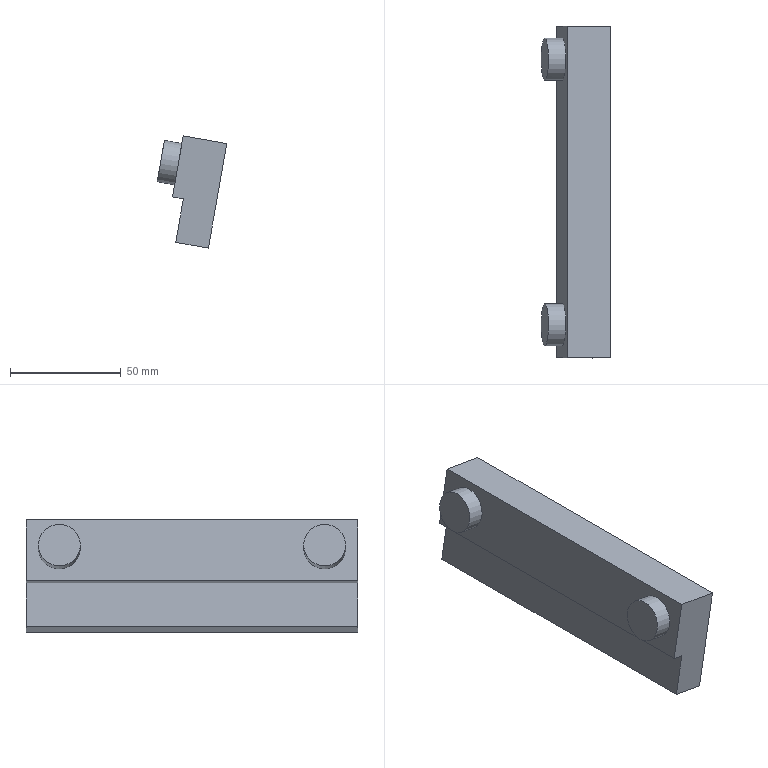Part | NX | features solid 2 | 1 solid | 12 faces | box 31.482 x 150 x 50.744 mm | volume 133536 mm3 | plane 10 | cylinder 2 | commonest cylinder face diameters 19 x2
STEP:
#1=CARTESIAN_POINT('',(-86.256,650.,343.869));
#2=VERTEX_POINT('',#1);
#3=CARTESIAN_POINT('',(-91.18,650.,344.737));
#4=VERTEX_POINT('',#3);
#5=CARTESIAN_POINT('',(-86.256,650.,343.869));
#6=DIRECTION('',(-0.9848,0.,0.1736));
#7=VECTOR('',#6,1000.);
#8=LINE('',#5,#7);
#9=EDGE_CURVE('',#2,#4,#8,.T.);
#10=ORIENTED_EDGE('',*,*,#9,.F.);
#11=CARTESIAN_POINT('',(-89.729,650.,324.172));
#12=VERTEX_POINT('',#11);
#13=CARTESIAN_POINT('',(-89.729,650.,324.172));
#14=DIRECTION('',(-0.1736,0.,-0.9848));
#15=VECTOR('',#14,1000.);
#16=LINE('',#13,#15);
#17=EDGE_CURVE('',#12,#2,#16,.F.);
#18=ORIENTED_EDGE('',*,*,#17,.F.);
#19=CARTESIAN_POINT('',(-74.957,650.,321.568));
#20=VERTEX_POINT('',#19);
#21=CARTESIAN_POINT('',(-74.957,650.,321.568));
#22=DIRECTION('',(-0.9848,0.,0.1736));
#23=VECTOR('',#22,1000.);
#24=LINE('',#21,#23);
#25=EDGE_CURVE('',#20,#12,#24,.T.);
#26=ORIENTED_EDGE('',*,*,#25,.F.);
#27=CARTESIAN_POINT('',(-66.622,650.,368.839));
#28=VERTEX_POINT('',#27);
#29=CARTESIAN_POINT('',(-75.304,650.,319.598));
#30=DIRECTION('',(0.1736,0.,0.9848));
#31=VECTOR('',#30,1000.);
#32=LINE('',#29,#31);
#33=EDGE_CURVE('',#20,#28,#32,.T.);
#34=ORIENTED_EDGE('',*,*,#33,.T.);
#35=CARTESIAN_POINT('',(-86.318,650.,372.311));
#36=VERTEX_POINT('',#35);
#37=CARTESIAN_POINT('',(-66.622,650.,368.839));
#38=DIRECTION('',(-0.9848,0.,0.1736));
#39=VECTOR('',#38,1000.);
#40=LINE('',#37,#39);
#41=EDGE_CURVE('',#28,#36,#40,.T.);
#42=ORIENTED_EDGE('',*,*,#41,.T.);
#43=CARTESIAN_POINT('',(-95.,650.,323.071));
#44=DIRECTION('',(0.1736,0.,0.9848));
#45=VECTOR('',#44,1000.);
#46=LINE('',#43,#45);
#47=EDGE_CURVE('',#4,#36,#46,.T.);
#48=ORIENTED_EDGE('',*,*,#47,.F.);
#49=EDGE_LOOP('',(#10,#18,#26,#34,#42,#48));
#50=FACE_BOUND('',#49,.T.);
#51=CARTESIAN_POINT('',(-75.304,650.,319.598));
#52=DIRECTION('',(0.,-1.,0.));
#53=DIRECTION('',(0.,0.,-1.));
#54=AXIS2_PLACEMENT_3D('',#51,#52,#53);
#55=PLANE('',#54);
#56=ADVANCED_FACE('',(#50),#55,.T.);
#57=CARTESIAN_POINT('',(-89.729,800.,324.172));
#58=VERTEX_POINT('',#57);
#59=CARTESIAN_POINT('',(-86.256,800.,343.869));
#60=VERTEX_POINT('',#59);
#61=CARTESIAN_POINT('',(-89.729,800.,324.172));
#62=DIRECTION('',(-0.1736,0.,-0.9848));
#63=VECTOR('',#62,1000.);
#64=LINE('',#61,#63);
#65=EDGE_CURVE('',#58,#60,#64,.F.);
#66=ORIENTED_EDGE('',*,*,#65,.T.);
#67=CARTESIAN_POINT('',(-91.18,800.,344.737));
#68=VERTEX_POINT('',#67);
#69=CARTESIAN_POINT('',(-86.256,800.,343.869));
#70=DIRECTION('',(-0.9848,0.,0.1736));
#71=VECTOR('',#70,1000.);
#72=LINE('',#69,#71);
#73=EDGE_CURVE('',#60,#68,#72,.T.);
#74=ORIENTED_EDGE('',*,*,#73,.T.);
#75=CARTESIAN_POINT('',(-86.318,800.,372.311));
#76=VERTEX_POINT('',#75);
#77=CARTESIAN_POINT('',(-95.,800.,323.071));
#78=DIRECTION('',(0.1736,0.,0.9848));
#79=VECTOR('',#78,1000.);
#80=LINE('',#77,#79);
#81=EDGE_CURVE('',#68,#76,#80,.T.);
#82=ORIENTED_EDGE('',*,*,#81,.T.);
#83=CARTESIAN_POINT('',(-66.622,800.,368.839));
#84=VERTEX_POINT('',#83);
#85=CARTESIAN_POINT('',(-66.622,800.,368.839));
#86=DIRECTION('',(-0.9848,0.,0.1736));
#87=VECTOR('',#86,1000.);
#88=LINE('',#85,#87);
#89=EDGE_CURVE('',#84,#76,#88,.T.);
#90=ORIENTED_EDGE('',*,*,#89,.F.);
#91=CARTESIAN_POINT('',(-74.957,800.,321.568));
#92=VERTEX_POINT('',#91);
#93=CARTESIAN_POINT('',(-75.304,800.,319.598));
#94=DIRECTION('',(0.1736,0.,0.9848));
#95=VECTOR('',#94,1000.);
#96=LINE('',#93,#95);
#97=EDGE_CURVE('',#92,#84,#96,.T.);
#98=ORIENTED_EDGE('',*,*,#97,.F.);
#99=CARTESIAN_POINT('',(-74.957,800.,321.568));
#100=DIRECTION('',(-0.9848,0.,0.1736));
#101=VECTOR('',#100,1000.);
#102=LINE('',#99,#101);
#103=EDGE_CURVE('',#92,#58,#102,.T.);
#104=ORIENTED_EDGE('',*,*,#103,.T.);
#105=EDGE_LOOP('',(#66,#74,#82,#90,#98,#104));
#106=FACE_BOUND('',#105,.T.);
#107=CARTESIAN_POINT('',(-75.304,800.,319.598));
#108=DIRECTION('',(0.,-1.,0.));
#109=DIRECTION('',(0.,0.,-1.));
#110=AXIS2_PLACEMENT_3D('',#107,#108,#109);
#111=PLANE('',#110);
#112=ADVANCED_FACE('',(#106),#111,.F.);
#113=ORIENTED_EDGE('',*,*,#25,.T.);
#114=CARTESIAN_POINT('',(-89.729,800.,324.172));
#115=DIRECTION('',(0.,-1.,0.));
#116=VECTOR('',#115,1000.);
#117=LINE('',#114,#116);
#118=EDGE_CURVE('',#58,#12,#117,.T.);
#119=ORIENTED_EDGE('',*,*,#118,.F.);
#120=ORIENTED_EDGE('',*,*,#103,.F.);
#121=CARTESIAN_POINT('',(-74.957,800.,321.568));
#122=DIRECTION('',(0.,-1.,0.));
#123=VECTOR('',#122,1000.);
#124=LINE('',#121,#123);
#125=EDGE_CURVE('',#92,#20,#124,.T.);
#126=ORIENTED_EDGE('',*,*,#125,.T.);
#127=EDGE_LOOP('',(#113,#119,#120,#126));
#128=FACE_BOUND('',#127,.T.);
#129=CARTESIAN_POINT('',(-74.957,800.,321.568));
#130=DIRECTION('',(-0.1736,0.,-0.9848));
#131=DIRECTION('',(-0.9848,0.,0.1736));
#132=AXIS2_PLACEMENT_3D('',#129,#130,#131);
#133=PLANE('',#132);
#134=ADVANCED_FACE('',(#128),#133,.T.);
#135=CARTESIAN_POINT('',(-86.926,665.,368.865));
#136=VERTEX_POINT('',#135);
#137=CARTESIAN_POINT('',(-88.575,665.,359.509));
#138=DIRECTION('',(-0.9848,0.,0.1736));
#139=DIRECTION('',(0.1736,0.,0.9848));
#140=AXIS2_PLACEMENT_3D('',#137,#138,#139);
#141=CIRCLE('',#140,9.5);
#142=EDGE_CURVE('',#136,#136,#141,.T.);
#143=ORIENTED_EDGE('',*,*,#142,.F.);
#144=EDGE_LOOP('',(#143));
#145=FACE_BOUND('',#144,.T.);
#146=CARTESIAN_POINT('',(-86.926,785.,368.865));
#147=VERTEX_POINT('',#146);
#148=CARTESIAN_POINT('',(-88.575,785.,359.509));
#149=DIRECTION('',(-0.9848,0.,0.1736));
#150=DIRECTION('',(0.1736,0.,0.9848));
#151=AXIS2_PLACEMENT_3D('',#148,#149,#150);
#152=CIRCLE('',#151,9.5);
#153=EDGE_CURVE('',#147,#147,#152,.T.);
#154=ORIENTED_EDGE('',*,*,#153,.F.);
#155=EDGE_LOOP('',(#154));
#156=FACE_BOUND('',#155,.T.);
#157=CARTESIAN_POINT('',(-91.18,800.,344.737));
#158=DIRECTION('',(0.,1.,0.));
#159=VECTOR('',#158,1000.);
#160=LINE('',#157,#159);
#161=EDGE_CURVE('',#68,#4,#160,.F.);
#162=ORIENTED_EDGE('',*,*,#161,.T.);
#163=ORIENTED_EDGE('',*,*,#47,.T.);
#164=CARTESIAN_POINT('',(-86.318,800.,372.311));
#165=DIRECTION('',(0.,-1.,0.));
#166=VECTOR('',#165,1000.);
#167=LINE('',#164,#166);
#168=EDGE_CURVE('',#76,#36,#167,.T.);
#169=ORIENTED_EDGE('',*,*,#168,.F.);
#170=ORIENTED_EDGE('',*,*,#81,.F.);
#171=EDGE_LOOP('',(#162,#163,#169,#170));
#172=FACE_BOUND('',#171,.T.);
#173=CARTESIAN_POINT('',(-95.,800.,323.071));
#174=DIRECTION('',(0.9848,0.,-0.1736));
#175=DIRECTION('',(-0.1736,0.,-0.9848));
#176=AXIS2_PLACEMENT_3D('',#173,#174,#175);
#177=PLANE('',#176);
#178=ADVANCED_FACE('',(#145,#156,#172),#177,.F.);
#179=ORIENTED_EDGE('',*,*,#168,.T.);
#180=ORIENTED_EDGE('',*,*,#41,.F.);
#181=CARTESIAN_POINT('',(-66.622,800.,368.839));
#182=DIRECTION('',(0.,-1.,0.));
#183=VECTOR('',#182,1000.);
#184=LINE('',#181,#183);
#185=EDGE_CURVE('',#84,#28,#184,.T.);
#186=ORIENTED_EDGE('',*,*,#185,.F.);
#187=ORIENTED_EDGE('',*,*,#89,.T.);
#188=EDGE_LOOP('',(#179,#180,#186,#187));
#189=FACE_BOUND('',#188,.T.);
#190=CARTESIAN_POINT('',(-66.622,800.,368.839));
#191=DIRECTION('',(-0.1736,0.,-0.9848));
#192=DIRECTION('',(-0.9848,0.,0.1736));
#193=AXIS2_PLACEMENT_3D('',#190,#191,#192);
#194=PLANE('',#193);
#195=ADVANCED_FACE('',(#189),#194,.F.);
#196=ORIENTED_EDGE('',*,*,#33,.F.);
#197=ORIENTED_EDGE('',*,*,#125,.F.);
#198=ORIENTED_EDGE('',*,*,#97,.T.);
#199=ORIENTED_EDGE('',*,*,#185,.T.);
#200=EDGE_LOOP('',(#196,#197,#198,#199));
#201=FACE_BOUND('',#200,.T.);
#202=CARTESIAN_POINT('',(-75.304,800.,319.598));
#203=DIRECTION('',(0.9848,0.,-0.1736));
#204=DIRECTION('',(-0.1736,0.,-0.9848));
#205=AXIS2_PLACEMENT_3D('',#202,#203,#204);
#206=PLANE('',#205);
#207=ADVANCED_FACE('',(#201),#206,.T.);
#208=CARTESIAN_POINT('',(-94.804,665.,370.254));
#209=VERTEX_POINT('',#208);
#210=CARTESIAN_POINT('',(-96.454,665.,360.898));
#211=DIRECTION('',(-0.9848,0.,0.1736));
#212=DIRECTION('',(0.1736,0.,0.9848));
#213=AXIS2_PLACEMENT_3D('',#210,#211,#212);
#214=CIRCLE('',#213,9.5);
#215=EDGE_CURVE('',#209,#209,#214,.T.);
#216=ORIENTED_EDGE('',*,*,#215,.T.);
#217=EDGE_LOOP('',(#216));
#218=FACE_BOUND('',#217,.T.);
#219=CARTESIAN_POINT('',(-96.454,665.,360.898));
#220=DIRECTION('',(-0.9848,0.,0.1736));
#221=DIRECTION('',(0.1736,0.,0.9848));
#222=AXIS2_PLACEMENT_3D('',#219,#220,#221);
#223=PLANE('',#222);
#224=ADVANCED_FACE('',(#218),#223,.T.);
#225=ORIENTED_EDGE('',*,*,#215,.F.);
#226=EDGE_LOOP('',(#225));
#227=FACE_BOUND('',#226,.T.);
#228=ORIENTED_EDGE('',*,*,#142,.T.);
#229=EDGE_LOOP('',(#228));
#230=FACE_BOUND('',#229,.T.);
#231=CARTESIAN_POINT('',(-88.575,665.,359.509));
#232=DIRECTION('',(-0.9848,0.,0.1736));
#233=DIRECTION('',(0.1736,0.,0.9848));
#234=AXIS2_PLACEMENT_3D('',#231,#232,#233);
#235=CYLINDRICAL_SURFACE('',#234,9.5);
#236=ADVANCED_FACE('',(#227,#230),#235,.T.);
#237=CARTESIAN_POINT('',(-94.804,785.,370.254));
#238=VERTEX_POINT('',#237);
#239=CARTESIAN_POINT('',(-96.454,785.,360.898));
#240=DIRECTION('',(-0.9848,0.,0.1736));
#241=DIRECTION('',(0.1736,0.,0.9848));
#242=AXIS2_PLACEMENT_3D('',#239,#240,#241);
#243=CIRCLE('',#242,9.5);
#244=EDGE_CURVE('',#238,#238,#243,.T.);
#245=ORIENTED_EDGE('',*,*,#244,.T.);
#246=EDGE_LOOP('',(#245));
#247=FACE_BOUND('',#246,.T.);
#248=CARTESIAN_POINT('',(-96.454,785.,360.898));
#249=DIRECTION('',(-0.9848,0.,0.1736));
#250=DIRECTION('',(0.1736,0.,0.9848));
#251=AXIS2_PLACEMENT_3D('',#248,#249,#250);
#252=PLANE('',#251);
#253=ADVANCED_FACE('',(#247),#252,.T.);
#254=ORIENTED_EDGE('',*,*,#244,.F.);
#255=EDGE_LOOP('',(#254));
#256=FACE_BOUND('',#255,.T.);
#257=ORIENTED_EDGE('',*,*,#153,.T.);
#258=EDGE_LOOP('',(#257));
#259=FACE_BOUND('',#258,.T.);
#260=CARTESIAN_POINT('',(-88.575,785.,359.509));
#261=DIRECTION('',(-0.9848,0.,0.1736));
#262=DIRECTION('',(0.1736,0.,0.9848));
#263=AXIS2_PLACEMENT_3D('',#260,#261,#262);
#264=CYLINDRICAL_SURFACE('',#263,9.5);
#265=ADVANCED_FACE('',(#256,#259),#264,.T.);
#266=ORIENTED_EDGE('',*,*,#65,.F.);
#267=ORIENTED_EDGE('',*,*,#118,.T.);
#268=ORIENTED_EDGE('',*,*,#17,.T.);
#269=CARTESIAN_POINT('',(-86.256,800.,343.869));
#270=DIRECTION('',(0.,1.,0.));
#271=VECTOR('',#270,1000.);
#272=LINE('',#269,#271);
#273=EDGE_CURVE('',#60,#2,#272,.F.);
#274=ORIENTED_EDGE('',*,*,#273,.F.);
#275=EDGE_LOOP('',(#266,#267,#268,#274));
#276=FACE_BOUND('',#275,.T.);
#277=CARTESIAN_POINT('',(-89.729,800.,324.172));
#278=DIRECTION('',(0.9848,0.,-0.1736));
#279=DIRECTION('',(0.,-1.,0.));
#280=AXIS2_PLACEMENT_3D('',#277,#278,#279);
#281=PLANE('',#280);
#282=ADVANCED_FACE('',(#276),#281,.F.);
#283=ORIENTED_EDGE('',*,*,#161,.F.);
#284=ORIENTED_EDGE('',*,*,#73,.F.);
#285=ORIENTED_EDGE('',*,*,#273,.T.);
#286=ORIENTED_EDGE('',*,*,#9,.T.);
#287=EDGE_LOOP('',(#283,#284,#285,#286));
#288=FACE_BOUND('',#287,.T.);
#289=CARTESIAN_POINT('',(-86.256,800.,343.869));
#290=DIRECTION('',(-0.1736,0.,-0.9848));
#291=DIRECTION('',(-0.9848,0.,0.1736));
#292=AXIS2_PLACEMENT_3D('',#289,#290,#291);
#293=PLANE('',#292);
#294=ADVANCED_FACE('',(#288),#293,.T.);
#295=CLOSED_SHELL('',(#56,#112,#134,#178,#195,#207,#224,#236,#253,#265,#282,#294));
#296=MANIFOLD_SOLID_BREP('',#295);
#297=(LENGTH_UNIT()NAMED_UNIT(*)SI_UNIT(.MILLI.,.METRE.));
#298=UNCERTAINTY_MEASURE_WITH_UNIT(LENGTH_MEASURE(0.00001),#297,'','');
#299=(NAMED_UNIT(*)PLANE_ANGLE_UNIT()SI_UNIT($,.RADIAN.));
#300=(NAMED_UNIT(*)SI_UNIT($,.STERADIAN.)SOLID_ANGLE_UNIT());
#301=(GEOMETRIC_REPRESENTATION_CONTEXT(3)GLOBAL_UNCERTAINTY_ASSIGNED_CONTEXT((#298))GLOBAL_UNIT_ASSIGNED_CONTEXT((#297,#299,#300))REPRESENTATION_CONTEXT('',''));
#302=ADVANCED_BREP_SHAPE_REPRESENTATION('',(#296),#301);